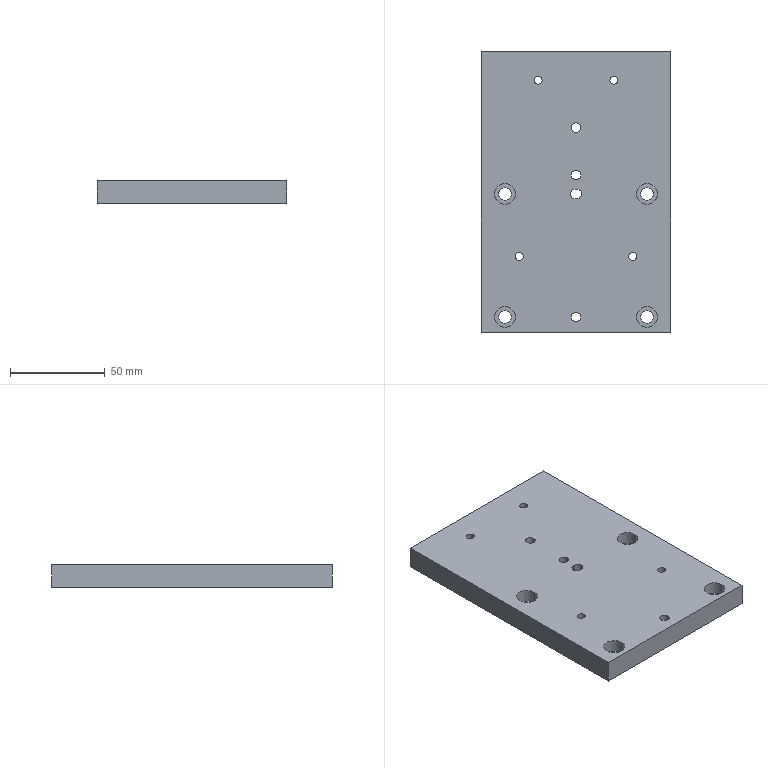Part | SolidWorks | features HoleWzd 6, Extrusion 1 | 1 solid | 45 faces | box 100 x 148 x 12 mm | volume 172636 mm3 | cylinder 33 | plane 12 | commonest cylinder face diameters 5 x9 4.2 x8 6.6 x8 11 x8
STEP:
#1=CARTESIAN_POINT('',(-32.1,-34.,0.));
#2=VERTEX_POINT('',#1);
#3=CARTESIAN_POINT('',(-27.9,-34.,0.));
#4=VERTEX_POINT('',#3);
#5=CARTESIAN_POINT('',(-30.,-34.,0.));
#6=DIRECTION('',(0.,0.,1.));
#7=DIRECTION('',(1.,0.,0.));
#8=AXIS2_PLACEMENT_3D('',#5,#6,#7);
#9=CIRCLE('',#8,2.1);
#10=EDGE_CURVE('',#2,#4,#9,.T.);
#11=ORIENTED_EDGE('',*,*,#10,.F.);
#12=CARTESIAN_POINT('',(-32.1,-34.,12.));
#13=VERTEX_POINT('',#12);
#14=CARTESIAN_POINT('',(-32.1,-34.,12.));
#15=DIRECTION('',(0.,0.,1.));
#16=VECTOR('',#15,1000.);
#17=LINE('',#14,#16);
#18=EDGE_CURVE('',#2,#13,#17,.T.);
#19=ORIENTED_EDGE('',*,*,#18,.T.);
#20=CARTESIAN_POINT('',(-27.9,-34.,12.));
#21=VERTEX_POINT('',#20);
#22=CARTESIAN_POINT('',(-30.,-34.,12.));
#23=DIRECTION('',(0.,0.,1.));
#24=DIRECTION('',(1.,0.,0.));
#25=AXIS2_PLACEMENT_3D('',#22,#23,#24);
#26=CIRCLE('',#25,2.1);
#27=EDGE_CURVE('',#13,#21,#26,.T.);
#28=ORIENTED_EDGE('',*,*,#27,.T.);
#29=CARTESIAN_POINT('',(-27.9,-34.,12.));
#30=DIRECTION('',(0.,0.,1.));
#31=VECTOR('',#30,1000.);
#32=LINE('',#29,#31);
#33=EDGE_CURVE('',#4,#21,#32,.T.);
#34=ORIENTED_EDGE('',*,*,#33,.F.);
#35=EDGE_LOOP('',(#11,#19,#28,#34));
#36=FACE_OUTER_BOUND('',#35,.T.);
#37=CARTESIAN_POINT('',(-30.,-34.,12.));
#38=DIRECTION('',(0.,0.,1.));
#39=DIRECTION('',(1.,0.,0.));
#40=AXIS2_PLACEMENT_3D('',#37,#38,#39);
#41=CYLINDRICAL_SURFACE('',#40,2.1);
#42=ADVANCED_FACE('',(#36),#41,.F.);
#43=CARTESIAN_POINT('',(27.9,-34.,0.));
#44=VERTEX_POINT('',#43);
#45=CARTESIAN_POINT('',(32.1,-34.,0.));
#46=VERTEX_POINT('',#45);
#47=CARTESIAN_POINT('',(30.,-34.,0.));
#48=DIRECTION('',(0.,0.,1.));
#49=DIRECTION('',(1.,0.,0.));
#50=AXIS2_PLACEMENT_3D('',#47,#48,#49);
#51=CIRCLE('',#50,2.1);
#52=EDGE_CURVE('',#44,#46,#51,.T.);
#53=ORIENTED_EDGE('',*,*,#52,.F.);
#54=CARTESIAN_POINT('',(27.9,-34.,12.));
#55=VERTEX_POINT('',#54);
#56=CARTESIAN_POINT('',(27.9,-34.,12.));
#57=DIRECTION('',(0.,0.,1.));
#58=VECTOR('',#57,1000.);
#59=LINE('',#56,#58);
#60=EDGE_CURVE('',#44,#55,#59,.T.);
#61=ORIENTED_EDGE('',*,*,#60,.T.);
#62=CARTESIAN_POINT('',(32.1,-34.,12.));
#63=VERTEX_POINT('',#62);
#64=CARTESIAN_POINT('',(30.,-34.,12.));
#65=DIRECTION('',(0.,0.,1.));
#66=DIRECTION('',(1.,0.,0.));
#67=AXIS2_PLACEMENT_3D('',#64,#65,#66);
#68=CIRCLE('',#67,2.1);
#69=EDGE_CURVE('',#55,#63,#68,.T.);
#70=ORIENTED_EDGE('',*,*,#69,.T.);
#71=CARTESIAN_POINT('',(32.1,-34.,12.));
#72=DIRECTION('',(0.,0.,1.));
#73=VECTOR('',#72,1000.);
#74=LINE('',#71,#73);
#75=EDGE_CURVE('',#46,#63,#74,.T.);
#76=ORIENTED_EDGE('',*,*,#75,.F.);
#77=EDGE_LOOP('',(#53,#61,#70,#76));
#78=FACE_OUTER_BOUND('',#77,.T.);
#79=CARTESIAN_POINT('',(30.,-34.,12.));
#80=DIRECTION('',(0.,0.,1.));
#81=DIRECTION('',(1.,0.,0.));
#82=AXIS2_PLACEMENT_3D('',#79,#80,#81);
#83=CYLINDRICAL_SURFACE('',#82,2.1);
#84=ADVANCED_FACE('',(#78),#83,.F.);
#85=CARTESIAN_POINT('',(-2.5,34.,0.));
#86=VERTEX_POINT('',#85);
#87=CARTESIAN_POINT('',(2.5,34.,0.));
#88=VERTEX_POINT('',#87);
#89=CARTESIAN_POINT('',(0.,34.,0.));
#90=DIRECTION('',(0.,0.,1.));
#91=DIRECTION('',(1.,0.,0.));
#92=AXIS2_PLACEMENT_3D('',#89,#90,#91);
#93=CIRCLE('',#92,2.5);
#94=EDGE_CURVE('',#86,#88,#93,.T.);
#95=ORIENTED_EDGE('',*,*,#94,.F.);
#96=CARTESIAN_POINT('',(-2.5,34.,12.));
#97=VERTEX_POINT('',#96);
#98=CARTESIAN_POINT('',(-2.5,34.,12.));
#99=DIRECTION('',(0.,0.,1.));
#100=VECTOR('',#99,1000.);
#101=LINE('',#98,#100);
#102=EDGE_CURVE('',#86,#97,#101,.T.);
#103=ORIENTED_EDGE('',*,*,#102,.T.);
#104=CARTESIAN_POINT('',(2.5,34.,12.));
#105=VERTEX_POINT('',#104);
#106=CARTESIAN_POINT('',(0.,34.,12.));
#107=DIRECTION('',(0.,0.,1.));
#108=DIRECTION('',(1.,0.,0.));
#109=AXIS2_PLACEMENT_3D('',#106,#107,#108);
#110=CIRCLE('',#109,2.5);
#111=EDGE_CURVE('',#97,#105,#110,.T.);
#112=ORIENTED_EDGE('',*,*,#111,.T.);
#113=CARTESIAN_POINT('',(2.5,34.,12.));
#114=DIRECTION('',(0.,0.,1.));
#115=VECTOR('',#114,1000.);
#116=LINE('',#113,#115);
#117=EDGE_CURVE('',#88,#105,#116,.T.);
#118=ORIENTED_EDGE('',*,*,#117,.F.);
#119=EDGE_LOOP('',(#95,#103,#112,#118));
#120=FACE_OUTER_BOUND('',#119,.T.);
#121=CARTESIAN_POINT('',(0.,34.,12.));
#122=DIRECTION('',(0.,0.,1.));
#123=DIRECTION('',(1.,0.,0.));
#124=AXIS2_PLACEMENT_3D('',#121,#122,#123);
#125=CYLINDRICAL_SURFACE('',#124,2.5);
#126=ADVANCED_FACE('',(#120),#125,.F.);
#127=CARTESIAN_POINT('',(-2.5,9.,0.));
#128=VERTEX_POINT('',#127);
#129=CARTESIAN_POINT('',(2.5,9.,0.));
#130=VERTEX_POINT('',#129);
#131=CARTESIAN_POINT('',(0.,9.,0.));
#132=DIRECTION('',(0.,0.,1.));
#133=DIRECTION('',(1.,0.,0.));
#134=AXIS2_PLACEMENT_3D('',#131,#132,#133);
#135=CIRCLE('',#134,2.5);
#136=EDGE_CURVE('',#128,#130,#135,.T.);
#137=ORIENTED_EDGE('',*,*,#136,.F.);
#138=CARTESIAN_POINT('',(-2.5,9.,12.));
#139=VERTEX_POINT('',#138);
#140=CARTESIAN_POINT('',(-2.5,9.,12.));
#141=DIRECTION('',(0.,0.,1.));
#142=VECTOR('',#141,1000.);
#143=LINE('',#140,#142);
#144=EDGE_CURVE('',#128,#139,#143,.T.);
#145=ORIENTED_EDGE('',*,*,#144,.T.);
#146=CARTESIAN_POINT('',(2.5,9.,12.));
#147=VERTEX_POINT('',#146);
#148=CARTESIAN_POINT('',(0.,9.,12.));
#149=DIRECTION('',(0.,0.,1.));
#150=DIRECTION('',(1.,0.,0.));
#151=AXIS2_PLACEMENT_3D('',#148,#149,#150);
#152=CIRCLE('',#151,2.5);
#153=EDGE_CURVE('',#139,#147,#152,.T.);
#154=ORIENTED_EDGE('',*,*,#153,.T.);
#155=CARTESIAN_POINT('',(2.5,9.,12.));
#156=DIRECTION('',(0.,0.,1.));
#157=VECTOR('',#156,1000.);
#158=LINE('',#155,#157);
#159=EDGE_CURVE('',#130,#147,#158,.T.);
#160=ORIENTED_EDGE('',*,*,#159,.F.);
#161=EDGE_LOOP('',(#137,#145,#154,#160));
#162=FACE_OUTER_BOUND('',#161,.T.);
#163=CARTESIAN_POINT('',(0.,9.,12.));
#164=DIRECTION('',(0.,0.,1.));
#165=DIRECTION('',(1.,0.,0.));
#166=AXIS2_PLACEMENT_3D('',#163,#164,#165);
#167=CYLINDRICAL_SURFACE('',#166,2.5);
#168=ADVANCED_FACE('',(#162),#167,.F.);
#169=CARTESIAN_POINT('',(22.1,59.,12.));
#170=VERTEX_POINT('',#169);
#171=CARTESIAN_POINT('',(17.9,59.,12.));
#172=VERTEX_POINT('',#171);
#173=CARTESIAN_POINT('',(20.,59.,12.));
#174=DIRECTION('',(0.,0.,-1.));
#175=DIRECTION('',(-1.,0.,0.));
#176=AXIS2_PLACEMENT_3D('',#173,#174,#175);
#177=CIRCLE('',#176,2.1);
#178=EDGE_CURVE('',#170,#172,#177,.T.);
#179=ORIENTED_EDGE('',*,*,#178,.F.);
#180=CARTESIAN_POINT('',(22.1,59.,0.));
#181=VERTEX_POINT('',#180);
#182=CARTESIAN_POINT('',(22.1,59.,0.));
#183=DIRECTION('',(0.,0.,-1.));
#184=VECTOR('',#183,1000.);
#185=LINE('',#182,#184);
#186=EDGE_CURVE('',#170,#181,#185,.T.);
#187=ORIENTED_EDGE('',*,*,#186,.T.);
#188=CARTESIAN_POINT('',(17.9,59.,0.));
#189=VERTEX_POINT('',#188);
#190=CARTESIAN_POINT('',(20.,59.,0.));
#191=DIRECTION('',(0.,0.,-1.));
#192=DIRECTION('',(-1.,0.,0.));
#193=AXIS2_PLACEMENT_3D('',#190,#191,#192);
#194=CIRCLE('',#193,2.1);
#195=EDGE_CURVE('',#181,#189,#194,.T.);
#196=ORIENTED_EDGE('',*,*,#195,.T.);
#197=CARTESIAN_POINT('',(17.9,59.,0.));
#198=DIRECTION('',(0.,0.,-1.));
#199=VECTOR('',#198,1000.);
#200=LINE('',#197,#199);
#201=EDGE_CURVE('',#172,#189,#200,.T.);
#202=ORIENTED_EDGE('',*,*,#201,.F.);
#203=EDGE_LOOP('',(#179,#187,#196,#202));
#204=FACE_OUTER_BOUND('',#203,.T.);
#205=CARTESIAN_POINT('',(20.,59.,0.));
#206=DIRECTION('',(0.,0.,-1.));
#207=DIRECTION('',(-1.,0.,0.));
#208=AXIS2_PLACEMENT_3D('',#205,#206,#207);
#209=CYLINDRICAL_SURFACE('',#208,2.1);
#210=ADVANCED_FACE('',(#204),#209,.F.);
#211=CARTESIAN_POINT('',(-17.9,59.,12.));
#212=VERTEX_POINT('',#211);
#213=CARTESIAN_POINT('',(-22.1,59.,12.));
#214=VERTEX_POINT('',#213);
#215=CARTESIAN_POINT('',(-20.,59.,12.));
#216=DIRECTION('',(0.,0.,-1.));
#217=DIRECTION('',(-1.,0.,0.));
#218=AXIS2_PLACEMENT_3D('',#215,#216,#217);
#219=CIRCLE('',#218,2.1);
#220=EDGE_CURVE('',#212,#214,#219,.T.);
#221=ORIENTED_EDGE('',*,*,#220,.F.);
#222=CARTESIAN_POINT('',(-17.9,59.,0.));
#223=VERTEX_POINT('',#222);
#224=CARTESIAN_POINT('',(-17.9,59.,0.));
#225=DIRECTION('',(0.,0.,-1.));
#226=VECTOR('',#225,1000.);
#227=LINE('',#224,#226);
#228=EDGE_CURVE('',#212,#223,#227,.T.);
#229=ORIENTED_EDGE('',*,*,#228,.T.);
#230=CARTESIAN_POINT('',(-22.1,59.,0.));
#231=VERTEX_POINT('',#230);
#232=CARTESIAN_POINT('',(-20.,59.,0.));
#233=DIRECTION('',(0.,0.,-1.));
#234=DIRECTION('',(-1.,0.,0.));
#235=AXIS2_PLACEMENT_3D('',#232,#233,#234);
#236=CIRCLE('',#235,2.1);
#237=EDGE_CURVE('',#223,#231,#236,.T.);
#238=ORIENTED_EDGE('',*,*,#237,.T.);
#239=CARTESIAN_POINT('',(-22.1,59.,0.));
#240=DIRECTION('',(0.,0.,-1.));
#241=VECTOR('',#240,1000.);
#242=LINE('',#239,#241);
#243=EDGE_CURVE('',#214,#231,#242,.T.);
#244=ORIENTED_EDGE('',*,*,#243,.F.);
#245=EDGE_LOOP('',(#221,#229,#238,#244));
#246=FACE_OUTER_BOUND('',#245,.T.);
#247=CARTESIAN_POINT('',(-20.,59.,0.));
#248=DIRECTION('',(0.,0.,-1.));
#249=DIRECTION('',(-1.,0.,0.));
#250=AXIS2_PLACEMENT_3D('',#247,#248,#249);
#251=CYLINDRICAL_SURFACE('',#250,2.1);
#252=ADVANCED_FACE('',(#246),#251,.F.);
#253=CARTESIAN_POINT('',(3.,-1.,0.));
#254=VERTEX_POINT('',#253);
#255=CARTESIAN_POINT('',(0.5,1.5,0.));
#256=VERTEX_POINT('',#255);
#257=CARTESIAN_POINT('',(0.5,-1.,0.));
#258=DIRECTION('',(0.,0.,1.));
#259=DIRECTION('',(1.,0.,0.));
#260=AXIS2_PLACEMENT_3D('',#257,#258,#259);
#261=CIRCLE('',#260,2.5);
#262=EDGE_CURVE('',#254,#256,#261,.T.);
#263=ORIENTED_EDGE('',*,*,#262,.F.);
#264=CARTESIAN_POINT('',(3.,-1.,12.));
#265=VERTEX_POINT('',#264);
#266=CARTESIAN_POINT('',(3.,-1.,12.));
#267=DIRECTION('',(0.,0.,1.));
#268=VECTOR('',#267,1000.);
#269=LINE('',#266,#268);
#270=EDGE_CURVE('',#254,#265,#269,.T.);
#271=ORIENTED_EDGE('',*,*,#270,.T.);
#272=CARTESIAN_POINT('',(0.5,1.5,12.));
#273=VERTEX_POINT('',#272);
#274=CARTESIAN_POINT('',(0.5,-1.,12.));
#275=DIRECTION('',(0.,0.,1.));
#276=DIRECTION('',(1.,0.,0.));
#277=AXIS2_PLACEMENT_3D('',#274,#275,#276);
#278=CIRCLE('',#277,2.5);
#279=EDGE_CURVE('',#265,#273,#278,.T.);
#280=ORIENTED_EDGE('',*,*,#279,.T.);
#281=CARTESIAN_POINT('',(0.5,1.5,12.));
#282=DIRECTION('',(0.,0.,1.));
#283=VECTOR('',#282,1000.);
#284=LINE('',#281,#283);
#285=EDGE_CURVE('',#256,#273,#284,.T.);
#286=ORIENTED_EDGE('',*,*,#285,.F.);
#287=EDGE_LOOP('',(#263,#271,#280,#286));
#288=FACE_OUTER_BOUND('',#287,.T.);
#289=CARTESIAN_POINT('',(0.5,-1.,12.));
#290=DIRECTION('',(0.,0.,1.));
#291=DIRECTION('',(1.,0.,0.));
#292=AXIS2_PLACEMENT_3D('',#289,#290,#291);
#293=CYLINDRICAL_SURFACE('',#292,2.5);
#294=ADVANCED_FACE('',(#288),#293,.F.);
#295=CARTESIAN_POINT('',(-2.5,-66.,0.));
#296=VERTEX_POINT('',#295);
#297=CARTESIAN_POINT('',(2.5,-66.,0.));
#298=VERTEX_POINT('',#297);
#299=CARTESIAN_POINT('',(0.,-66.,0.));
#300=DIRECTION('',(0.,0.,1.));
#301=DIRECTION('',(1.,0.,0.));
#302=AXIS2_PLACEMENT_3D('',#299,#300,#301);
#303=CIRCLE('',#302,2.5);
#304=EDGE_CURVE('',#296,#298,#303,.T.);
#305=ORIENTED_EDGE('',*,*,#304,.F.);
#306=CARTESIAN_POINT('',(-2.5,-66.,12.));
#307=VERTEX_POINT('',#306);
#308=CARTESIAN_POINT('',(-2.5,-66.,12.));
#309=DIRECTION('',(0.,0.,1.));
#310=VECTOR('',#309,1000.);
#311=LINE('',#308,#310);
#312=EDGE_CURVE('',#296,#307,#311,.T.);
#313=ORIENTED_EDGE('',*,*,#312,.T.);
#314=CARTESIAN_POINT('',(2.5,-66.,12.));
#315=VERTEX_POINT('',#314);
#316=CARTESIAN_POINT('',(0.,-66.,12.));
#317=DIRECTION('',(0.,0.,1.));
#318=DIRECTION('',(1.,0.,0.));
#319=AXIS2_PLACEMENT_3D('',#316,#317,#318);
#320=CIRCLE('',#319,2.5);
#321=EDGE_CURVE('',#307,#315,#320,.T.);
#322=ORIENTED_EDGE('',*,*,#321,.T.);
#323=CARTESIAN_POINT('',(2.5,-66.,12.));
#324=DIRECTION('',(0.,0.,1.));
#325=VECTOR('',#324,1000.);
#326=LINE('',#323,#325);
#327=EDGE_CURVE('',#298,#315,#326,.T.);
#328=ORIENTED_EDGE('',*,*,#327,.F.);
#329=EDGE_LOOP('',(#305,#313,#322,#328));
#330=FACE_OUTER_BOUND('',#329,.T.);
#331=CARTESIAN_POINT('',(0.,-66.,12.));
#332=DIRECTION('',(0.,0.,1.));
#333=DIRECTION('',(1.,0.,0.));
#334=AXIS2_PLACEMENT_3D('',#331,#332,#333);
#335=CYLINDRICAL_SURFACE('',#334,2.5);
#336=ADVANCED_FACE('',(#330),#335,.F.);
#337=CARTESIAN_POINT('',(-43.,-1.,5.2));
#338=VERTEX_POINT('',#337);
#339=CARTESIAN_POINT('',(-32.,-1.,5.2));
#340=VERTEX_POINT('',#339);
#341=CARTESIAN_POINT('',(-37.5,-1.,5.2));
#342=DIRECTION('',(0.,0.,1.));
#343=DIRECTION('',(1.,0.,0.));
#344=AXIS2_PLACEMENT_3D('',#341,#342,#343);
#345=CIRCLE('',#344,5.5);
#346=EDGE_CURVE('',#338,#340,#345,.T.);
#347=ORIENTED_EDGE('',*,*,#346,.F.);
#348=CARTESIAN_POINT('',(-43.,-1.,12.));
#349=VERTEX_POINT('',#348);
#350=CARTESIAN_POINT('',(-43.,-1.,12.));
#351=DIRECTION('',(0.,0.,1.));
#352=VECTOR('',#351,1000.);
#353=LINE('',#350,#352);
#354=EDGE_CURVE('',#338,#349,#353,.T.);
#355=ORIENTED_EDGE('',*,*,#354,.T.);
#356=CARTESIAN_POINT('',(-32.,-1.,12.));
#357=VERTEX_POINT('',#356);
#358=CARTESIAN_POINT('',(-37.5,-1.,12.));
#359=DIRECTION('',(0.,0.,1.));
#360=DIRECTION('',(1.,0.,0.));
#361=AXIS2_PLACEMENT_3D('',#358,#359,#360);
#362=CIRCLE('',#361,5.5);
#363=EDGE_CURVE('',#349,#357,#362,.T.);
#364=ORIENTED_EDGE('',*,*,#363,.T.);
#365=CARTESIAN_POINT('',(-32.,-1.,12.));
#366=DIRECTION('',(0.,0.,1.));
#367=VECTOR('',#366,1000.);
#368=LINE('',#365,#367);
#369=EDGE_CURVE('',#340,#357,#368,.T.);
#370=ORIENTED_EDGE('',*,*,#369,.F.);
#371=EDGE_LOOP('',(#347,#355,#364,#370));
#372=FACE_OUTER_BOUND('',#371,.T.);
#373=CARTESIAN_POINT('',(-37.5,-1.,12.));
#374=DIRECTION('',(0.,0.,1.));
#375=DIRECTION('',(1.,0.,0.));
#376=AXIS2_PLACEMENT_3D('',#373,#374,#375);
#377=CYLINDRICAL_SURFACE('',#376,5.5);
#378=ADVANCED_FACE('',(#372),#377,.F.);
#379=CARTESIAN_POINT('',(-40.8,-1.,0.));
#380=VERTEX_POINT('',#379);
#381=CARTESIAN_POINT('',(-34.2,-1.,0.));
#382=VERTEX_POINT('',#381);
#383=CARTESIAN_POINT('',(-37.5,-1.,0.));
#384=DIRECTION('',(0.,0.,1.));
#385=DIRECTION('',(1.,0.,0.));
#386=AXIS2_PLACEMENT_3D('',#383,#384,#385);
#387=CIRCLE('',#386,3.3);
#388=EDGE_CURVE('',#380,#382,#387,.T.);
#389=ORIENTED_EDGE('',*,*,#388,.F.);
#390=CARTESIAN_POINT('',(-40.8,-1.,5.2));
#391=VERTEX_POINT('',#390);
#392=CARTESIAN_POINT('',(-40.8,-1.,12.));
#393=DIRECTION('',(0.,0.,1.));
#394=VECTOR('',#393,1000.);
#395=LINE('',#392,#394);
#396=EDGE_CURVE('',#380,#391,#395,.T.);
#397=ORIENTED_EDGE('',*,*,#396,.T.);
#398=CARTESIAN_POINT('',(-34.2,-1.,5.2));
#399=VERTEX_POINT('',#398);
#400=CARTESIAN_POINT('',(-37.5,-1.,5.2));
#401=DIRECTION('',(0.,0.,1.));
#402=DIRECTION('',(1.,0.,0.));
#403=AXIS2_PLACEMENT_3D('',#400,#401,#402);
#404=CIRCLE('',#403,3.3);
#405=EDGE_CURVE('',#391,#399,#404,.T.);
#406=ORIENTED_EDGE('',*,*,#405,.T.);
#407=CARTESIAN_POINT('',(-34.2,-1.,12.));
#408=DIRECTION('',(0.,0.,1.));
#409=VECTOR('',#408,1000.);
#410=LINE('',#407,#409);
#411=EDGE_CURVE('',#382,#399,#410,.T.);
#412=ORIENTED_EDGE('',*,*,#411,.F.);
#413=EDGE_LOOP('',(#389,#397,#406,#412));
#414=FACE_OUTER_BOUND('',#413,.T.);
#415=CARTESIAN_POINT('',(-37.5,-1.,12.));
#416=DIRECTION('',(0.,0.,1.));
#417=DIRECTION('',(1.,0.,0.));
#418=AXIS2_PLACEMENT_3D('',#415,#416,#417);
#419=CYLINDRICAL_SURFACE('',#418,3.3);
#420=ADVANCED_FACE('',(#414),#419,.F.);
#421=CARTESIAN_POINT('',(-43.,-66.,5.2));
#422=VERTEX_POINT('',#421);
#423=CARTESIAN_POINT('',(-32.,-66.,5.2));
#424=VERTEX_POINT('',#423);
#425=CARTESIAN_POINT('',(-37.5,-66.,5.2));
#426=DIRECTION('',(0.,0.,1.));
#427=DIRECTION('',(1.,0.,0.));
#428=AXIS2_PLACEMENT_3D('',#425,#426,#427);
#429=CIRCLE('',#428,5.5);
#430=EDGE_CURVE('',#422,#424,#429,.T.);
#431=ORIENTED_EDGE('',*,*,#430,.F.);
#432=CARTESIAN_POINT('',(-43.,-66.,12.));
#433=VERTEX_POINT('',#432);
#434=CARTESIAN_POINT('',(-43.,-66.,12.));
#435=DIRECTION('',(0.,0.,1.));
#436=VECTOR('',#435,1000.);
#437=LINE('',#434,#436);
#438=EDGE_CURVE('',#422,#433,#437,.T.);
#439=ORIENTED_EDGE('',*,*,#438,.T.);
#440=CARTESIAN_POINT('',(-32.,-66.,12.));
#441=VERTEX_POINT('',#440);
#442=CARTESIAN_POINT('',(-37.5,-66.,12.));
#443=DIRECTION('',(0.,0.,1.));
#444=DIRECTION('',(1.,0.,0.));
#445=AXIS2_PLACEMENT_3D('',#442,#443,#444);
#446=CIRCLE('',#445,5.5);
#447=EDGE_CURVE('',#433,#441,#446,.T.);
#448=ORIENTED_EDGE('',*,*,#447,.T.);
#449=CARTESIAN_POINT('',(-32.,-66.,12.));
#450=DIRECTION('',(0.,0.,1.));
#451=VECTOR('',#450,1000.);
#452=LINE('',#449,#451);
#453=EDGE_CURVE('',#424,#441,#452,.T.);
#454=ORIENTED_EDGE('',*,*,#453,.F.);
#455=EDGE_LOOP('',(#431,#439,#448,#454));
#456=FACE_OUTER_BOUND('',#455,.T.);
#457=CARTESIAN_POINT('',(-37.5,-66.,12.));
#458=DIRECTION('',(0.,0.,1.));
#459=DIRECTION('',(1.,0.,0.));
#460=AXIS2_PLACEMENT_3D('',#457,#458,#459);
#461=CYLINDRICAL_SURFACE('',#460,5.5);
#462=ADVANCED_FACE('',(#456),#461,.F.);
#463=CARTESIAN_POINT('',(-40.8,-66.,0.));
#464=VERTEX_POINT('',#463);
#465=CARTESIAN_POINT('',(-34.2,-66.,0.));
#466=VERTEX_POINT('',#465);
#467=CARTESIAN_POINT('',(-37.5,-66.,0.));
#468=DIRECTION('',(0.,0.,1.));
#469=DIRECTION('',(1.,0.,0.));
#470=AXIS2_PLACEMENT_3D('',#467,#468,#469);
#471=CIRCLE('',#470,3.3);
#472=EDGE_CURVE('',#464,#466,#471,.T.);
#473=ORIENTED_EDGE('',*,*,#472,.F.);
#474=CARTESIAN_POINT('',(-40.8,-66.,5.2));
#475=VERTEX_POINT('',#474);
#476=CARTESIAN_POINT('',(-40.8,-66.,12.));
#477=DIRECTION('',(0.,0.,1.));
#478=VECTOR('',#477,1000.);
#479=LINE('',#476,#478);
#480=EDGE_CURVE('',#464,#475,#479,.T.);
#481=ORIENTED_EDGE('',*,*,#480,.T.);
#482=CARTESIAN_POINT('',(-34.2,-66.,5.2));
#483=VERTEX_POINT('',#482);
#484=CARTESIAN_POINT('',(-37.5,-66.,5.2));
#485=DIRECTION('',(0.,0.,1.));
#486=DIRECTION('',(1.,0.,0.));
#487=AXIS2_PLACEMENT_3D('',#484,#485,#486);
#488=CIRCLE('',#487,3.3);
#489=EDGE_CURVE('',#475,#483,#488,.T.);
#490=ORIENTED_EDGE('',*,*,#489,.T.);
#491=CARTESIAN_POINT('',(-34.2,-66.,12.));
#492=DIRECTION('',(0.,0.,1.));
#493=VECTOR('',#492,1000.);
#494=LINE('',#491,#493);
#495=EDGE_CURVE('',#466,#483,#494,.T.);
#496=ORIENTED_EDGE('',*,*,#495,.F.);
#497=EDGE_LOOP('',(#473,#481,#490,#496));
#498=FACE_OUTER_BOUND('',#497,.T.);
#499=CARTESIAN_POINT('',(-37.5,-66.,12.));
#500=DIRECTION('',(0.,0.,1.));
#501=DIRECTION('',(1.,0.,0.));
#502=AXIS2_PLACEMENT_3D('',#499,#500,#501);
#503=CYLINDRICAL_SURFACE('',#502,3.3);
#504=ADVANCED_FACE('',(#498),#503,.F.);
#505=CARTESIAN_POINT('',(32.,-1.,5.2));
#506=VERTEX_POINT('',#505);
#507=CARTESIAN_POINT('',(43.,-1.,5.2));
#508=VERTEX_POINT('',#507);
#509=CARTESIAN_POINT('',(37.5,-1.,5.2));
#510=DIRECTION('',(0.,0.,1.));
#511=DIRECTION('',(1.,0.,0.));
#512=AXIS2_PLACEMENT_3D('',#509,#510,#511);
#513=CIRCLE('',#512,5.5);
#514=EDGE_CURVE('',#506,#508,#513,.T.);
#515=ORIENTED_EDGE('',*,*,#514,.F.);
#516=CARTESIAN_POINT('',(32.,-1.,12.));
#517=VERTEX_POINT('',#516);
#518=CARTESIAN_POINT('',(32.,-1.,12.));
#519=DIRECTION('',(0.,0.,1.));
#520=VECTOR('',#519,1000.);
#521=LINE('',#518,#520);
#522=EDGE_CURVE('',#506,#517,#521,.T.);
#523=ORIENTED_EDGE('',*,*,#522,.T.);
#524=CARTESIAN_POINT('',(43.,-1.,12.));
#525=VERTEX_POINT('',#524);
#526=CARTESIAN_POINT('',(37.5,-1.,12.));
#527=DIRECTION('',(0.,0.,1.));
#528=DIRECTION('',(1.,0.,0.));
#529=AXIS2_PLACEMENT_3D('',#526,#527,#528);
#530=CIRCLE('',#529,5.5);
#531=EDGE_CURVE('',#517,#525,#530,.T.);
#532=ORIENTED_EDGE('',*,*,#531,.T.);
#533=CARTESIAN_POINT('',(43.,-1.,12.));
#534=DIRECTION('',(0.,0.,1.));
#535=VECTOR('',#534,1000.);
#536=LINE('',#533,#535);
#537=EDGE_CURVE('',#508,#525,#536,.T.);
#538=ORIENTED_EDGE('',*,*,#537,.F.);
#539=EDGE_LOOP('',(#515,#523,#532,#538));
#540=FACE_OUTER_BOUND('',#539,.T.);
#541=CARTESIAN_POINT('',(37.5,-1.,12.));
#542=DIRECTION('',(0.,0.,1.));
#543=DIRECTION('',(1.,0.,0.));
#544=AXIS2_PLACEMENT_3D('',#541,#542,#543);
#545=CYLINDRICAL_SURFACE('',#544,5.5);
#546=ADVANCED_FACE('',(#540),#545,.F.);
#547=CARTESIAN_POINT('',(34.2,-1.,0.));
#548=VERTEX_POINT('',#547);
#549=CARTESIAN_POINT('',(40.8,-1.,0.));
#550=VERTEX_POINT('',#549);
#551=CARTESIAN_POINT('',(37.5,-1.,0.));
#552=DIRECTION('',(0.,0.,1.));
#553=DIRECTION('',(1.,0.,0.));
#554=AXIS2_PLACEMENT_3D('',#551,#552,#553);
#555=CIRCLE('',#554,3.3);
#556=EDGE_CURVE('',#548,#550,#555,.T.);
#557=ORIENTED_EDGE('',*,*,#556,.F.);
#558=CARTESIAN_POINT('',(34.2,-1.,5.2));
#559=VERTEX_POINT('',#558);
#560=CARTESIAN_POINT('',(34.2,-1.,12.));
#561=DIRECTION('',(0.,0.,1.));
#562=VECTOR('',#561,1000.);
#563=LINE('',#560,#562);
#564=EDGE_CURVE('',#548,#559,#563,.T.);
#565=ORIENTED_EDGE('',*,*,#564,.T.);
#566=CARTESIAN_POINT('',(40.8,-1.,5.2));
#567=VERTEX_POINT('',#566);
#568=CARTESIAN_POINT('',(37.5,-1.,5.2));
#569=DIRECTION('',(0.,0.,1.));
#570=DIRECTION('',(1.,0.,0.));
#571=AXIS2_PLACEMENT_3D('',#568,#569,#570);
#572=CIRCLE('',#571,3.3);
#573=EDGE_CURVE('',#559,#567,#572,.T.);
#574=ORIENTED_EDGE('',*,*,#573,.T.);
#575=CARTESIAN_POINT('',(40.8,-1.,12.));
#576=DIRECTION('',(0.,0.,1.));
#577=VECTOR('',#576,1000.);
#578=LINE('',#575,#577);
#579=EDGE_CURVE('',#550,#567,#578,.T.);
#580=ORIENTED_EDGE('',*,*,#579,.F.);
#581=EDGE_LOOP('',(#557,#565,#574,#580));
#582=FACE_OUTER_BOUND('',#581,.T.);
#583=CARTESIAN_POINT('',(37.5,-1.,12.));
#584=DIRECTION('',(0.,0.,1.));
#585=DIRECTION('',(1.,0.,0.));
#586=AXIS2_PLACEMENT_3D('',#583,#584,#585);
#587=CYLINDRICAL_SURFACE('',#586,3.3);
#588=ADVANCED_FACE('',(#582),#587,.F.);
#589=CARTESIAN_POINT('',(32.,-66.,5.2));
#590=VERTEX_POINT('',#589);
#591=CARTESIAN_POINT('',(43.,-66.,5.2));
#592=VERTEX_POINT('',#591);
#593=CARTESIAN_POINT('',(37.5,-66.,5.2));
#594=DIRECTION('',(0.,0.,1.));
#595=DIRECTION('',(1.,0.,0.));
#596=AXIS2_PLACEMENT_3D('',#593,#594,#595);
#597=CIRCLE('',#596,5.5);
#598=EDGE_CURVE('',#590,#592,#597,.T.);
#599=ORIENTED_EDGE('',*,*,#598,.F.);
#600=CARTESIAN_POINT('',(32.,-66.,12.));
#601=VERTEX_POINT('',#600);
#602=CARTESIAN_POINT('',(32.,-66.,12.));
#603=DIRECTION('',(0.,0.,1.));
#604=VECTOR('',#603,1000.);
#605=LINE('',#602,#604);
#606=EDGE_CURVE('',#590,#601,#605,.T.);
#607=ORIENTED_EDGE('',*,*,#606,.T.);
#608=CARTESIAN_POINT('',(43.,-66.,12.));
#609=VERTEX_POINT('',#608);
#610=CARTESIAN_POINT('',(37.5,-66.,12.));
#611=DIRECTION('',(0.,0.,1.));
#612=DIRECTION('',(1.,0.,0.));
#613=AXIS2_PLACEMENT_3D('',#610,#611,#612);
#614=CIRCLE('',#613,5.5);
#615=EDGE_CURVE('',#601,#609,#614,.T.);
#616=ORIENTED_EDGE('',*,*,#615,.T.);
#617=CARTESIAN_POINT('',(43.,-66.,12.));
#618=DIRECTION('',(0.,0.,1.));
#619=VECTOR('',#618,1000.);
#620=LINE('',#617,#619);
#621=EDGE_CURVE('',#592,#609,#620,.T.);
#622=ORIENTED_EDGE('',*,*,#621,.F.);
#623=EDGE_LOOP('',(#599,#607,#616,#622));
#624=FACE_OUTER_BOUND('',#623,.T.);
#625=CARTESIAN_POINT('',(37.5,-66.,12.));
#626=DIRECTION('',(0.,0.,1.));
#627=DIRECTION('',(1.,0.,0.));
#628=AXIS2_PLACEMENT_3D('',#625,#626,#627);
#629=CYLINDRICAL_SURFACE('',#628,5.5);
#630=ADVANCED_FACE('',(#624),#629,.F.);
#631=CARTESIAN_POINT('',(34.2,-66.,0.));
#632=VERTEX_POINT('',#631);
#633=CARTESIAN_POINT('',(40.8,-66.,0.));
#634=VERTEX_POINT('',#633);
#635=CARTESIAN_POINT('',(37.5,-66.,0.));
#636=DIRECTION('',(0.,0.,1.));
#637=DIRECTION('',(1.,0.,0.));
#638=AXIS2_PLACEMENT_3D('',#635,#636,#637);
#639=CIRCLE('',#638,3.3);
#640=EDGE_CURVE('',#632,#634,#639,.T.);
#641=ORIENTED_EDGE('',*,*,#640,.F.);
#642=CARTESIAN_POINT('',(34.2,-66.,5.2));
#643=VERTEX_POINT('',#642);
#644=CARTESIAN_POINT('',(34.2,-66.,12.));
#645=DIRECTION('',(0.,0.,1.));
#646=VECTOR('',#645,1000.);
#647=LINE('',#644,#646);
#648=EDGE_CURVE('',#632,#643,#647,.T.);
#649=ORIENTED_EDGE('',*,*,#648,.T.);
#650=CARTESIAN_POINT('',(40.8,-66.,5.2));
#651=VERTEX_POINT('',#650);
#652=CARTESIAN_POINT('',(37.5,-66.,5.2));
#653=DIRECTION('',(0.,0.,1.));
#654=DIRECTION('',(1.,0.,0.));
#655=AXIS2_PLACEMENT_3D('',#652,#653,#654);
#656=CIRCLE('',#655,3.3);
#657=EDGE_CURVE('',#643,#651,#656,.T.);
#658=ORIENTED_EDGE('',*,*,#657,.T.);
#659=CARTESIAN_POINT('',(40.8,-66.,12.));
#660=DIRECTION('',(0.,0.,1.));
#661=VECTOR('',#660,1000.);
#662=LINE('',#659,#661);
#663=EDGE_CURVE('',#634,#651,#662,.T.);
#664=ORIENTED_EDGE('',*,*,#663,.F.);
#665=EDGE_LOOP('',(#641,#649,#658,#664));
#666=FACE_OUTER_BOUND('',#665,.T.);
#667=CARTESIAN_POINT('',(37.5,-66.,12.));
#668=DIRECTION('',(0.,0.,1.));
#669=DIRECTION('',(1.,0.,0.));
#670=AXIS2_PLACEMENT_3D('',#667,#668,#669);
#671=CYLINDRICAL_SURFACE('',#670,3.3);
#672=ADVANCED_FACE('',(#666),#671,.F.);
#673=CARTESIAN_POINT('',(50.,-74.,0.));
#674=VERTEX_POINT('',#673);
#675=CARTESIAN_POINT('',(50.,74.,0.));
#676=VERTEX_POINT('',#675);
#677=CARTESIAN_POINT('',(50.,74.,0.));
#678=DIRECTION('',(0.,1.,0.));
#679=VECTOR('',#678,1000.);
#680=LINE('',#677,#679);
#681=EDGE_CURVE('',#674,#676,#680,.T.);
#682=ORIENTED_EDGE('',*,*,#681,.T.);
#683=CARTESIAN_POINT('',(50.,74.,12.));
#684=VERTEX_POINT('',#683);
#685=CARTESIAN_POINT('',(50.,74.,12.));
#686=DIRECTION('',(0.,0.,-1.));
#687=VECTOR('',#686,1000.);
#688=LINE('',#685,#687);
#689=EDGE_CURVE('',#684,#676,#688,.T.);
#690=ORIENTED_EDGE('',*,*,#689,.F.);
#691=CARTESIAN_POINT('',(50.,-74.,12.));
#692=VERTEX_POINT('',#691);
#693=CARTESIAN_POINT('',(50.,74.,12.));
#694=DIRECTION('',(0.,1.,0.));
#695=VECTOR('',#694,1000.);
#696=LINE('',#693,#695);
#697=EDGE_CURVE('',#692,#684,#696,.T.);
#698=ORIENTED_EDGE('',*,*,#697,.F.);
#699=CARTESIAN_POINT('',(50.,-74.,12.));
#700=DIRECTION('',(0.,0.,-1.));
#701=VECTOR('',#700,1000.);
#702=LINE('',#699,#701);
#703=EDGE_CURVE('',#692,#674,#702,.T.);
#704=ORIENTED_EDGE('',*,*,#703,.T.);
#705=EDGE_LOOP('',(#682,#690,#698,#704));
#706=FACE_OUTER_BOUND('',#705,.T.);
#707=CARTESIAN_POINT('',(50.,74.,12.));
#708=DIRECTION('',(-1.,0.,0.));
#709=DIRECTION('',(0.,-1.,0.));
#710=AXIS2_PLACEMENT_3D('',#707,#708,#709);
#711=PLANE('',#710);
#712=ADVANCED_FACE('',(#706),#711,.F.);
#713=CARTESIAN_POINT('',(-50.,74.,0.));
#714=VERTEX_POINT('',#713);
#715=CARTESIAN_POINT('',(-50.,74.,0.));
#716=DIRECTION('',(-1.,0.,0.));
#717=VECTOR('',#716,1000.);
#718=LINE('',#715,#717);
#719=EDGE_CURVE('',#676,#714,#718,.T.);
#720=ORIENTED_EDGE('',*,*,#719,.T.);
#721=CARTESIAN_POINT('',(-50.,74.,12.));
#722=VERTEX_POINT('',#721);
#723=CARTESIAN_POINT('',(-50.,74.,12.));
#724=DIRECTION('',(0.,0.,-1.));
#725=VECTOR('',#724,1000.);
#726=LINE('',#723,#725);
#727=EDGE_CURVE('',#722,#714,#726,.T.);
#728=ORIENTED_EDGE('',*,*,#727,.F.);
#729=CARTESIAN_POINT('',(-50.,74.,12.));
#730=DIRECTION('',(-1.,0.,0.));
#731=VECTOR('',#730,1000.);
#732=LINE('',#729,#731);
#733=EDGE_CURVE('',#684,#722,#732,.T.);
#734=ORIENTED_EDGE('',*,*,#733,.F.);
#735=ORIENTED_EDGE('',*,*,#689,.T.);
#736=EDGE_LOOP('',(#720,#728,#734,#735));
#737=FACE_OUTER_BOUND('',#736,.T.);
#738=CARTESIAN_POINT('',(-50.,74.,12.));
#739=DIRECTION('',(0.,-1.,0.));
#740=DIRECTION('',(1.,0.,0.));
#741=AXIS2_PLACEMENT_3D('',#738,#739,#740);
#742=PLANE('',#741);
#743=ADVANCED_FACE('',(#737),#742,.F.);
#744=CARTESIAN_POINT('',(-50.,-74.,0.));
#745=VERTEX_POINT('',#744);
#746=CARTESIAN_POINT('',(-50.,74.,0.));
#747=DIRECTION('',(0.,-1.,0.));
#748=VECTOR('',#747,1000.);
#749=LINE('',#746,#748);
#750=EDGE_CURVE('',#714,#745,#749,.T.);
#751=ORIENTED_EDGE('',*,*,#750,.T.);
#752=CARTESIAN_POINT('',(-50.,-74.,12.));
#753=VERTEX_POINT('',#752);
#754=CARTESIAN_POINT('',(-50.,-74.,12.));
#755=DIRECTION('',(0.,0.,-1.));
#756=VECTOR('',#755,1000.);
#757=LINE('',#754,#756);
#758=EDGE_CURVE('',#753,#745,#757,.T.);
#759=ORIENTED_EDGE('',*,*,#758,.F.);
#760=CARTESIAN_POINT('',(-50.,74.,12.));
#761=DIRECTION('',(0.,-1.,0.));
#762=VECTOR('',#761,1000.);
#763=LINE('',#760,#762);
#764=EDGE_CURVE('',#722,#753,#763,.T.);
#765=ORIENTED_EDGE('',*,*,#764,.F.);
#766=ORIENTED_EDGE('',*,*,#727,.T.);
#767=EDGE_LOOP('',(#751,#759,#765,#766));
#768=FACE_OUTER_BOUND('',#767,.T.);
#769=CARTESIAN_POINT('',(-50.,74.,12.));
#770=DIRECTION('',(1.,0.,0.));
#771=DIRECTION('',(0.,0.,-1.));
#772=AXIS2_PLACEMENT_3D('',#769,#770,#771);
#773=PLANE('',#772);
#774=ADVANCED_FACE('',(#768),#773,.F.);
#775=CARTESIAN_POINT('',(-50.,-74.,0.));
#776=DIRECTION('',(1.,0.,0.));
#777=VECTOR('',#776,1000.);
#778=LINE('',#775,#777);
#779=EDGE_CURVE('',#745,#674,#778,.T.);
#780=ORIENTED_EDGE('',*,*,#779,.T.);
#781=ORIENTED_EDGE('',*,*,#703,.F.);
#782=CARTESIAN_POINT('',(-50.,-74.,12.));
#783=DIRECTION('',(1.,0.,0.));
#784=VECTOR('',#783,1000.);
#785=LINE('',#782,#784);
#786=EDGE_CURVE('',#753,#692,#785,.T.);
#787=ORIENTED_EDGE('',*,*,#786,.F.);
#788=ORIENTED_EDGE('',*,*,#758,.T.);
#789=EDGE_LOOP('',(#780,#781,#787,#788));
#790=FACE_OUTER_BOUND('',#789,.T.);
#791=CARTESIAN_POINT('',(-50.,-74.,12.));
#792=DIRECTION('',(0.,1.,0.));
#793=DIRECTION('',(-1.,0.,0.));
#794=AXIS2_PLACEMENT_3D('',#791,#792,#793);
#795=PLANE('',#794);
#796=ADVANCED_FACE('',(#790),#795,.F.);
#797=CARTESIAN_POINT('',(-30.,-34.,12.));
#798=DIRECTION('',(0.,0.,1.));
#799=DIRECTION('',(1.,0.,0.));
#800=AXIS2_PLACEMENT_3D('',#797,#798,#799);
#801=CIRCLE('',#800,2.1);
#802=EDGE_CURVE('',#21,#13,#801,.T.);
#803=ORIENTED_EDGE('',*,*,#802,.F.);
#804=ORIENTED_EDGE('',*,*,#27,.F.);
#805=EDGE_LOOP('',(#803,#804));
#806=FACE_BOUND('',#805,.T.);
#807=CARTESIAN_POINT('',(30.,-34.,12.));
#808=DIRECTION('',(0.,0.,1.));
#809=DIRECTION('',(1.,0.,0.));
#810=AXIS2_PLACEMENT_3D('',#807,#808,#809);
#811=CIRCLE('',#810,2.1);
#812=EDGE_CURVE('',#63,#55,#811,.T.);
#813=ORIENTED_EDGE('',*,*,#812,.F.);
#814=ORIENTED_EDGE('',*,*,#69,.F.);
#815=EDGE_LOOP('',(#813,#814));
#816=FACE_BOUND('',#815,.T.);
#817=CARTESIAN_POINT('',(0.,34.,12.));
#818=DIRECTION('',(0.,0.,1.));
#819=DIRECTION('',(1.,0.,0.));
#820=AXIS2_PLACEMENT_3D('',#817,#818,#819);
#821=CIRCLE('',#820,2.5);
#822=EDGE_CURVE('',#105,#97,#821,.T.);
#823=ORIENTED_EDGE('',*,*,#822,.F.);
#824=ORIENTED_EDGE('',*,*,#111,.F.);
#825=EDGE_LOOP('',(#823,#824));
#826=FACE_BOUND('',#825,.T.);
#827=CARTESIAN_POINT('',(0.,9.,12.));
#828=DIRECTION('',(0.,0.,1.));
#829=DIRECTION('',(1.,0.,0.));
#830=AXIS2_PLACEMENT_3D('',#827,#828,#829);
#831=CIRCLE('',#830,2.5);
#832=EDGE_CURVE('',#147,#139,#831,.T.);
#833=ORIENTED_EDGE('',*,*,#832,.F.);
#834=ORIENTED_EDGE('',*,*,#153,.F.);
#835=EDGE_LOOP('',(#833,#834));
#836=FACE_BOUND('',#835,.T.);
#837=CARTESIAN_POINT('',(20.,59.,12.));
#838=DIRECTION('',(0.,0.,-1.));
#839=DIRECTION('',(-1.,0.,0.));
#840=AXIS2_PLACEMENT_3D('',#837,#838,#839);
#841=CIRCLE('',#840,2.1);
#842=EDGE_CURVE('',#172,#170,#841,.T.);
#843=ORIENTED_EDGE('',*,*,#842,.T.);
#844=ORIENTED_EDGE('',*,*,#178,.T.);
#845=EDGE_LOOP('',(#843,#844));
#846=FACE_BOUND('',#845,.T.);
#847=CARTESIAN_POINT('',(-20.,59.,12.));
#848=DIRECTION('',(0.,0.,-1.));
#849=DIRECTION('',(-1.,0.,0.));
#850=AXIS2_PLACEMENT_3D('',#847,#848,#849);
#851=CIRCLE('',#850,2.1);
#852=EDGE_CURVE('',#214,#212,#851,.T.);
#853=ORIENTED_EDGE('',*,*,#852,.T.);
#854=ORIENTED_EDGE('',*,*,#220,.T.);
#855=EDGE_LOOP('',(#853,#854));
#856=FACE_BOUND('',#855,.T.);
#857=CARTESIAN_POINT('',(-0.5,-3.5,12.));
#858=VERTEX_POINT('',#857);
#859=CARTESIAN_POINT('',(0.5,-3.5,12.));
#860=VERTEX_POINT('',#859);
#861=CARTESIAN_POINT('',(-0.5,-3.5,12.));
#862=DIRECTION('',(1.,0.,0.));
#863=VECTOR('',#862,1000.);
#864=LINE('',#861,#863);
#865=EDGE_CURVE('',#858,#860,#864,.T.);
#866=ORIENTED_EDGE('',*,*,#865,.F.);
#867=CARTESIAN_POINT('',(-0.5,1.5,12.));
#868=VERTEX_POINT('',#867);
#869=CARTESIAN_POINT('',(-0.5,-1.,12.));
#870=DIRECTION('',(0.,0.,1.));
#871=DIRECTION('',(1.,0.,0.));
#872=AXIS2_PLACEMENT_3D('',#869,#870,#871);
#873=CIRCLE('',#872,2.5);
#874=EDGE_CURVE('',#868,#858,#873,.T.);
#875=ORIENTED_EDGE('',*,*,#874,.F.);
#876=CARTESIAN_POINT('',(-0.5,1.5,12.));
#877=DIRECTION('',(1.,0.,0.));
#878=VECTOR('',#877,1000.);
#879=LINE('',#876,#878);
#880=EDGE_CURVE('',#868,#273,#879,.T.);
#881=ORIENTED_EDGE('',*,*,#880,.T.);
#882=ORIENTED_EDGE('',*,*,#279,.F.);
#883=CARTESIAN_POINT('',(0.5,-1.,12.));
#884=DIRECTION('',(0.,0.,1.));
#885=DIRECTION('',(1.,0.,0.));
#886=AXIS2_PLACEMENT_3D('',#883,#884,#885);
#887=CIRCLE('',#886,2.5);
#888=EDGE_CURVE('',#860,#265,#887,.T.);
#889=ORIENTED_EDGE('',*,*,#888,.F.);
#890=EDGE_LOOP('',(#866,#875,#881,#882,#889));
#891=FACE_BOUND('',#890,.T.);
#892=CARTESIAN_POINT('',(0.,-66.,12.));
#893=DIRECTION('',(0.,0.,1.));
#894=DIRECTION('',(1.,0.,0.));
#895=AXIS2_PLACEMENT_3D('',#892,#893,#894);
#896=CIRCLE('',#895,2.5);
#897=EDGE_CURVE('',#315,#307,#896,.T.);
#898=ORIENTED_EDGE('',*,*,#897,.F.);
#899=ORIENTED_EDGE('',*,*,#321,.F.);
#900=EDGE_LOOP('',(#898,#899));
#901=FACE_BOUND('',#900,.T.);
#902=CARTESIAN_POINT('',(-37.5,-1.,12.));
#903=DIRECTION('',(0.,0.,1.));
#904=DIRECTION('',(1.,0.,0.));
#905=AXIS2_PLACEMENT_3D('',#902,#903,#904);
#906=CIRCLE('',#905,5.5);
#907=EDGE_CURVE('',#357,#349,#906,.T.);
#908=ORIENTED_EDGE('',*,*,#907,.F.);
#909=ORIENTED_EDGE('',*,*,#363,.F.);
#910=EDGE_LOOP('',(#908,#909));
#911=FACE_BOUND('',#910,.T.);
#912=CARTESIAN_POINT('',(-37.5,-66.,12.));
#913=DIRECTION('',(0.,0.,1.));
#914=DIRECTION('',(1.,0.,0.));
#915=AXIS2_PLACEMENT_3D('',#912,#913,#914);
#916=CIRCLE('',#915,5.5);
#917=EDGE_CURVE('',#441,#433,#916,.T.);
#918=ORIENTED_EDGE('',*,*,#917,.F.);
#919=ORIENTED_EDGE('',*,*,#447,.F.);
#920=EDGE_LOOP('',(#918,#919));
#921=FACE_BOUND('',#920,.T.);
#922=CARTESIAN_POINT('',(37.5,-1.,12.));
#923=DIRECTION('',(0.,0.,1.));
#924=DIRECTION('',(1.,0.,0.));
#925=AXIS2_PLACEMENT_3D('',#922,#923,#924);
#926=CIRCLE('',#925,5.5);
#927=EDGE_CURVE('',#525,#517,#926,.T.);
#928=ORIENTED_EDGE('',*,*,#927,.F.);
#929=ORIENTED_EDGE('',*,*,#531,.F.);
#930=EDGE_LOOP('',(#928,#929));
#931=FACE_BOUND('',#930,.T.);
#932=CARTESIAN_POINT('',(37.5,-66.,12.));
#933=DIRECTION('',(0.,0.,1.));
#934=DIRECTION('',(1.,0.,0.));
#935=AXIS2_PLACEMENT_3D('',#932,#933,#934);
#936=CIRCLE('',#935,5.5);
#937=EDGE_CURVE('',#609,#601,#936,.T.);
#938=ORIENTED_EDGE('',*,*,#937,.F.);
#939=ORIENTED_EDGE('',*,*,#615,.F.);
#940=EDGE_LOOP('',(#938,#939));
#941=FACE_BOUND('',#940,.T.);
#942=ORIENTED_EDGE('',*,*,#697,.T.);
#943=ORIENTED_EDGE('',*,*,#733,.T.);
#944=ORIENTED_EDGE('',*,*,#764,.T.);
#945=ORIENTED_EDGE('',*,*,#786,.T.);
#946=EDGE_LOOP('',(#942,#943,#944,#945));
#947=FACE_OUTER_BOUND('',#946,.T.);
#948=CARTESIAN_POINT('',(0.,0.,12.));
#949=DIRECTION('',(0.,0.,1.));
#950=DIRECTION('',(1.,0.,0.));
#951=AXIS2_PLACEMENT_3D('',#948,#949,#950);
#952=PLANE('',#951);
#953=ADVANCED_FACE('',(#806,#816,#826,#836,#846,#856,#891,#901,#911,#921,#931,#941,#947),#952,.T.);
#954=CARTESIAN_POINT('',(-30.,-34.,0.));
#955=DIRECTION('',(0.,0.,1.));
#956=DIRECTION('',(1.,0.,0.));
#957=AXIS2_PLACEMENT_3D('',#954,#955,#956);
#958=CIRCLE('',#957,2.1);
#959=EDGE_CURVE('',#4,#2,#958,.T.);
#960=ORIENTED_EDGE('',*,*,#959,.T.);
#961=ORIENTED_EDGE('',*,*,#10,.T.);
#962=EDGE_LOOP('',(#960,#961));
#963=FACE_BOUND('',#962,.T.);
#964=CARTESIAN_POINT('',(30.,-34.,0.));
#965=DIRECTION('',(0.,0.,1.));
#966=DIRECTION('',(1.,0.,0.));
#967=AXIS2_PLACEMENT_3D('',#964,#965,#966);
#968=CIRCLE('',#967,2.1);
#969=EDGE_CURVE('',#46,#44,#968,.T.);
#970=ORIENTED_EDGE('',*,*,#969,.T.);
#971=ORIENTED_EDGE('',*,*,#52,.T.);
#972=EDGE_LOOP('',(#970,#971));
#973=FACE_BOUND('',#972,.T.);
#974=CARTESIAN_POINT('',(0.,34.,0.));
#975=DIRECTION('',(0.,0.,1.));
#976=DIRECTION('',(1.,0.,0.));
#977=AXIS2_PLACEMENT_3D('',#974,#975,#976);
#978=CIRCLE('',#977,2.5);
#979=EDGE_CURVE('',#88,#86,#978,.T.);
#980=ORIENTED_EDGE('',*,*,#979,.T.);
#981=ORIENTED_EDGE('',*,*,#94,.T.);
#982=EDGE_LOOP('',(#980,#981));
#983=FACE_BOUND('',#982,.T.);
#984=CARTESIAN_POINT('',(0.,9.,0.));
#985=DIRECTION('',(0.,0.,1.));
#986=DIRECTION('',(1.,0.,0.));
#987=AXIS2_PLACEMENT_3D('',#984,#985,#986);
#988=CIRCLE('',#987,2.5);
#989=EDGE_CURVE('',#130,#128,#988,.T.);
#990=ORIENTED_EDGE('',*,*,#989,.T.);
#991=ORIENTED_EDGE('',*,*,#136,.T.);
#992=EDGE_LOOP('',(#990,#991));
#993=FACE_BOUND('',#992,.T.);
#994=CARTESIAN_POINT('',(20.,59.,0.));
#995=DIRECTION('',(0.,0.,-1.));
#996=DIRECTION('',(-1.,0.,0.));
#997=AXIS2_PLACEMENT_3D('',#994,#995,#996);
#998=CIRCLE('',#997,2.1);
#999=EDGE_CURVE('',#189,#181,#998,.T.);
#1000=ORIENTED_EDGE('',*,*,#999,.F.);
#1001=ORIENTED_EDGE('',*,*,#195,.F.);
#1002=EDGE_LOOP('',(#1000,#1001));
#1003=FACE_BOUND('',#1002,.T.);
#1004=CARTESIAN_POINT('',(-20.,59.,0.));
#1005=DIRECTION('',(0.,0.,-1.));
#1006=DIRECTION('',(-1.,0.,0.));
#1007=AXIS2_PLACEMENT_3D('',#1004,#1005,#1006);
#1008=CIRCLE('',#1007,2.1);
#1009=EDGE_CURVE('',#231,#223,#1008,.T.);
#1010=ORIENTED_EDGE('',*,*,#1009,.F.);
#1011=ORIENTED_EDGE('',*,*,#237,.F.);
#1012=EDGE_LOOP('',(#1010,#1011));
#1013=FACE_BOUND('',#1012,.T.);
#1014=CARTESIAN_POINT('',(0.5,-3.5,0.));
#1015=VERTEX_POINT('',#1014);
#1016=CARTESIAN_POINT('',(0.5,-1.,0.));
#1017=DIRECTION('',(0.,0.,1.));
#1018=DIRECTION('',(1.,0.,0.));
#1019=AXIS2_PLACEMENT_3D('',#1016,#1017,#1018);
#1020=CIRCLE('',#1019,2.5);
#1021=EDGE_CURVE('',#1015,#254,#1020,.T.);
#1022=ORIENTED_EDGE('',*,*,#1021,.T.);
#1023=ORIENTED_EDGE('',*,*,#262,.T.);
#1024=CARTESIAN_POINT('',(-0.5,1.5,0.));
#1025=VERTEX_POINT('',#1024);
#1026=CARTESIAN_POINT('',(0.,1.5,0.));
#1027=DIRECTION('',(-1.,0.,0.));
#1028=VECTOR('',#1027,1000.);
#1029=LINE('',#1026,#1028);
#1030=EDGE_CURVE('',#256,#1025,#1029,.T.);
#1031=ORIENTED_EDGE('',*,*,#1030,.T.);
#1032=CARTESIAN_POINT('',(-0.5,-3.5,0.));
#1033=VERTEX_POINT('',#1032);
#1034=CARTESIAN_POINT('',(-0.5,-1.,0.));
#1035=DIRECTION('',(0.,0.,1.));
#1036=DIRECTION('',(1.,0.,0.));
#1037=AXIS2_PLACEMENT_3D('',#1034,#1035,#1036);
#1038=CIRCLE('',#1037,2.5);
#1039=EDGE_CURVE('',#1025,#1033,#1038,.T.);
#1040=ORIENTED_EDGE('',*,*,#1039,.T.);
#1041=CARTESIAN_POINT('',(0.,-3.5,0.));
#1042=DIRECTION('',(1.,0.,0.));
#1043=VECTOR('',#1042,1000.);
#1044=LINE('',#1041,#1043);
#1045=EDGE_CURVE('',#1033,#1015,#1044,.T.);
#1046=ORIENTED_EDGE('',*,*,#1045,.T.);
#1047=EDGE_LOOP('',(#1022,#1023,#1031,#1040,#1046));
#1048=FACE_BOUND('',#1047,.T.);
#1049=CARTESIAN_POINT('',(0.,-66.,0.));
#1050=DIRECTION('',(0.,0.,1.));
#1051=DIRECTION('',(1.,0.,0.));
#1052=AXIS2_PLACEMENT_3D('',#1049,#1050,#1051);
#1053=CIRCLE('',#1052,2.5);
#1054=EDGE_CURVE('',#298,#296,#1053,.T.);
#1055=ORIENTED_EDGE('',*,*,#1054,.T.);
#1056=ORIENTED_EDGE('',*,*,#304,.T.);
#1057=EDGE_LOOP('',(#1055,#1056));
#1058=FACE_BOUND('',#1057,.T.);
#1059=CARTESIAN_POINT('',(-37.5,-1.,0.));
#1060=DIRECTION('',(0.,0.,1.));
#1061=DIRECTION('',(1.,0.,0.));
#1062=AXIS2_PLACEMENT_3D('',#1059,#1060,#1061);
#1063=CIRCLE('',#1062,3.3);
#1064=EDGE_CURVE('',#382,#380,#1063,.T.);
#1065=ORIENTED_EDGE('',*,*,#1064,.T.);
#1066=ORIENTED_EDGE('',*,*,#388,.T.);
#1067=EDGE_LOOP('',(#1065,#1066));
#1068=FACE_BOUND('',#1067,.T.);
#1069=CARTESIAN_POINT('',(-37.5,-66.,0.));
#1070=DIRECTION('',(0.,0.,1.));
#1071=DIRECTION('',(1.,0.,0.));
#1072=AXIS2_PLACEMENT_3D('',#1069,#1070,#1071);
#1073=CIRCLE('',#1072,3.3);
#1074=EDGE_CURVE('',#466,#464,#1073,.T.);
#1075=ORIENTED_EDGE('',*,*,#1074,.T.);
#1076=ORIENTED_EDGE('',*,*,#472,.T.);
#1077=EDGE_LOOP('',(#1075,#1076));
#1078=FACE_BOUND('',#1077,.T.);
#1079=CARTESIAN_POINT('',(37.5,-1.,0.));
#1080=DIRECTION('',(0.,0.,1.));
#1081=DIRECTION('',(1.,0.,0.));
#1082=AXIS2_PLACEMENT_3D('',#1079,#1080,#1081);
#1083=CIRCLE('',#1082,3.3);
#1084=EDGE_CURVE('',#550,#548,#1083,.T.);
#1085=ORIENTED_EDGE('',*,*,#1084,.T.);
#1086=ORIENTED_EDGE('',*,*,#556,.T.);
#1087=EDGE_LOOP('',(#1085,#1086));
#1088=FACE_BOUND('',#1087,.T.);
#1089=CARTESIAN_POINT('',(37.5,-66.,0.));
#1090=DIRECTION('',(0.,0.,1.));
#1091=DIRECTION('',(1.,0.,0.));
#1092=AXIS2_PLACEMENT_3D('',#1089,#1090,#1091);
#1093=CIRCLE('',#1092,3.3);
#1094=EDGE_CURVE('',#634,#632,#1093,.T.);
#1095=ORIENTED_EDGE('',*,*,#1094,.T.);
#1096=ORIENTED_EDGE('',*,*,#640,.T.);
#1097=EDGE_LOOP('',(#1095,#1096));
#1098=FACE_BOUND('',#1097,.T.);
#1099=ORIENTED_EDGE('',*,*,#681,.F.);
#1100=ORIENTED_EDGE('',*,*,#779,.F.);
#1101=ORIENTED_EDGE('',*,*,#750,.F.);
#1102=ORIENTED_EDGE('',*,*,#719,.F.);
#1103=EDGE_LOOP('',(#1099,#1100,#1101,#1102));
#1104=FACE_OUTER_BOUND('',#1103,.T.);
#1105=CARTESIAN_POINT('',(0.,0.,0.));
#1106=DIRECTION('',(0.,0.,1.));
#1107=DIRECTION('',(1.,0.,0.));
#1108=AXIS2_PLACEMENT_3D('',#1105,#1106,#1107);
#1109=PLANE('',#1108);
#1110=ADVANCED_FACE('',(#963,#973,#983,#993,#1003,#1013,#1048,#1058,#1068,#1078,#1088,#1098,#1104),#1109,.F.);
#1111=ORIENTED_EDGE('',*,*,#648,.F.);
#1112=ORIENTED_EDGE('',*,*,#1094,.F.);
#1113=ORIENTED_EDGE('',*,*,#663,.T.);
#1114=CARTESIAN_POINT('',(37.5,-66.,5.2));
#1115=DIRECTION('',(0.,0.,1.));
#1116=DIRECTION('',(1.,0.,0.));
#1117=AXIS2_PLACEMENT_3D('',#1114,#1115,#1116);
#1118=CIRCLE('',#1117,3.3);
#1119=EDGE_CURVE('',#651,#643,#1118,.T.);
#1120=ORIENTED_EDGE('',*,*,#1119,.T.);
#1121=EDGE_LOOP('',(#1111,#1112,#1113,#1120));
#1122=FACE_OUTER_BOUND('',#1121,.T.);
#1123=CARTESIAN_POINT('',(37.5,-66.,12.));
#1124=DIRECTION('',(0.,0.,1.));
#1125=DIRECTION('',(1.,0.,0.));
#1126=AXIS2_PLACEMENT_3D('',#1123,#1124,#1125);
#1127=CYLINDRICAL_SURFACE('',#1126,3.3);
#1128=ADVANCED_FACE('',(#1122),#1127,.F.);
#1129=ORIENTED_EDGE('',*,*,#1119,.F.);
#1130=ORIENTED_EDGE('',*,*,#657,.F.);
#1131=EDGE_LOOP('',(#1129,#1130));
#1132=FACE_BOUND('',#1131,.T.);
#1133=CARTESIAN_POINT('',(37.5,-66.,5.2));
#1134=DIRECTION('',(0.,0.,1.));
#1135=DIRECTION('',(1.,0.,0.));
#1136=AXIS2_PLACEMENT_3D('',#1133,#1134,#1135);
#1137=CIRCLE('',#1136,5.5);
#1138=EDGE_CURVE('',#592,#590,#1137,.T.);
#1139=ORIENTED_EDGE('',*,*,#1138,.T.);
#1140=ORIENTED_EDGE('',*,*,#598,.T.);
#1141=EDGE_LOOP('',(#1139,#1140));
#1142=FACE_OUTER_BOUND('',#1141,.T.);
#1143=CARTESIAN_POINT('',(40.8,-66.,5.2));
#1144=DIRECTION('',(0.,0.,-1.));
#1145=DIRECTION('',(-1.,0.,0.));
#1146=AXIS2_PLACEMENT_3D('',#1143,#1144,#1145);
#1147=PLANE('',#1146);
#1148=ADVANCED_FACE('',(#1132,#1142),#1147,.F.);
#1149=ORIENTED_EDGE('',*,*,#606,.F.);
#1150=ORIENTED_EDGE('',*,*,#1138,.F.);
#1151=ORIENTED_EDGE('',*,*,#621,.T.);
#1152=ORIENTED_EDGE('',*,*,#937,.T.);
#1153=EDGE_LOOP('',(#1149,#1150,#1151,#1152));
#1154=FACE_OUTER_BOUND('',#1153,.T.);
#1155=CARTESIAN_POINT('',(37.5,-66.,12.));
#1156=DIRECTION('',(0.,0.,1.));
#1157=DIRECTION('',(1.,0.,0.));
#1158=AXIS2_PLACEMENT_3D('',#1155,#1156,#1157);
#1159=CYLINDRICAL_SURFACE('',#1158,5.5);
#1160=ADVANCED_FACE('',(#1154),#1159,.F.);
#1161=ORIENTED_EDGE('',*,*,#564,.F.);
#1162=ORIENTED_EDGE('',*,*,#1084,.F.);
#1163=ORIENTED_EDGE('',*,*,#579,.T.);
#1164=CARTESIAN_POINT('',(37.5,-1.,5.2));
#1165=DIRECTION('',(0.,0.,1.));
#1166=DIRECTION('',(1.,0.,0.));
#1167=AXIS2_PLACEMENT_3D('',#1164,#1165,#1166);
#1168=CIRCLE('',#1167,3.3);
#1169=EDGE_CURVE('',#567,#559,#1168,.T.);
#1170=ORIENTED_EDGE('',*,*,#1169,.T.);
#1171=EDGE_LOOP('',(#1161,#1162,#1163,#1170));
#1172=FACE_OUTER_BOUND('',#1171,.T.);
#1173=CARTESIAN_POINT('',(37.5,-1.,12.));
#1174=DIRECTION('',(0.,0.,1.));
#1175=DIRECTION('',(1.,0.,0.));
#1176=AXIS2_PLACEMENT_3D('',#1173,#1174,#1175);
#1177=CYLINDRICAL_SURFACE('',#1176,3.3);
#1178=ADVANCED_FACE('',(#1172),#1177,.F.);
#1179=ORIENTED_EDGE('',*,*,#1169,.F.);
#1180=ORIENTED_EDGE('',*,*,#573,.F.);
#1181=EDGE_LOOP('',(#1179,#1180));
#1182=FACE_BOUND('',#1181,.T.);
#1183=CARTESIAN_POINT('',(37.5,-1.,5.2));
#1184=DIRECTION('',(0.,0.,1.));
#1185=DIRECTION('',(1.,0.,0.));
#1186=AXIS2_PLACEMENT_3D('',#1183,#1184,#1185);
#1187=CIRCLE('',#1186,5.5);
#1188=EDGE_CURVE('',#508,#506,#1187,.T.);
#1189=ORIENTED_EDGE('',*,*,#1188,.T.);
#1190=ORIENTED_EDGE('',*,*,#514,.T.);
#1191=EDGE_LOOP('',(#1189,#1190));
#1192=FACE_OUTER_BOUND('',#1191,.T.);
#1193=CARTESIAN_POINT('',(40.8,-1.,5.2));
#1194=DIRECTION('',(0.,0.,-1.));
#1195=DIRECTION('',(-1.,0.,0.));
#1196=AXIS2_PLACEMENT_3D('',#1193,#1194,#1195);
#1197=PLANE('',#1196);
#1198=ADVANCED_FACE('',(#1182,#1192),#1197,.F.);
#1199=ORIENTED_EDGE('',*,*,#522,.F.);
#1200=ORIENTED_EDGE('',*,*,#1188,.F.);
#1201=ORIENTED_EDGE('',*,*,#537,.T.);
#1202=ORIENTED_EDGE('',*,*,#927,.T.);
#1203=EDGE_LOOP('',(#1199,#1200,#1201,#1202));
#1204=FACE_OUTER_BOUND('',#1203,.T.);
#1205=CARTESIAN_POINT('',(37.5,-1.,12.));
#1206=DIRECTION('',(0.,0.,1.));
#1207=DIRECTION('',(1.,0.,0.));
#1208=AXIS2_PLACEMENT_3D('',#1205,#1206,#1207);
#1209=CYLINDRICAL_SURFACE('',#1208,5.5);
#1210=ADVANCED_FACE('',(#1204),#1209,.F.);
#1211=ORIENTED_EDGE('',*,*,#480,.F.);
#1212=ORIENTED_EDGE('',*,*,#1074,.F.);
#1213=ORIENTED_EDGE('',*,*,#495,.T.);
#1214=CARTESIAN_POINT('',(-37.5,-66.,5.2));
#1215=DIRECTION('',(0.,0.,1.));
#1216=DIRECTION('',(1.,0.,0.));
#1217=AXIS2_PLACEMENT_3D('',#1214,#1215,#1216);
#1218=CIRCLE('',#1217,3.3);
#1219=EDGE_CURVE('',#483,#475,#1218,.T.);
#1220=ORIENTED_EDGE('',*,*,#1219,.T.);
#1221=EDGE_LOOP('',(#1211,#1212,#1213,#1220));
#1222=FACE_OUTER_BOUND('',#1221,.T.);
#1223=CARTESIAN_POINT('',(-37.5,-66.,12.));
#1224=DIRECTION('',(0.,0.,1.));
#1225=DIRECTION('',(1.,0.,0.));
#1226=AXIS2_PLACEMENT_3D('',#1223,#1224,#1225);
#1227=CYLINDRICAL_SURFACE('',#1226,3.3);
#1228=ADVANCED_FACE('',(#1222),#1227,.F.);
#1229=ORIENTED_EDGE('',*,*,#1219,.F.);
#1230=ORIENTED_EDGE('',*,*,#489,.F.);
#1231=EDGE_LOOP('',(#1229,#1230));
#1232=FACE_BOUND('',#1231,.T.);
#1233=CARTESIAN_POINT('',(-37.5,-66.,5.2));
#1234=DIRECTION('',(0.,0.,1.));
#1235=DIRECTION('',(1.,0.,0.));
#1236=AXIS2_PLACEMENT_3D('',#1233,#1234,#1235);
#1237=CIRCLE('',#1236,5.5);
#1238=EDGE_CURVE('',#424,#422,#1237,.T.);
#1239=ORIENTED_EDGE('',*,*,#1238,.T.);
#1240=ORIENTED_EDGE('',*,*,#430,.T.);
#1241=EDGE_LOOP('',(#1239,#1240));
#1242=FACE_OUTER_BOUND('',#1241,.T.);
#1243=CARTESIAN_POINT('',(-34.2,-66.,5.2));
#1244=DIRECTION('',(0.,0.,-1.));
#1245=DIRECTION('',(-1.,0.,0.));
#1246=AXIS2_PLACEMENT_3D('',#1243,#1244,#1245);
#1247=PLANE('',#1246);
#1248=ADVANCED_FACE('',(#1232,#1242),#1247,.F.);
#1249=ORIENTED_EDGE('',*,*,#438,.F.);
#1250=ORIENTED_EDGE('',*,*,#1238,.F.);
#1251=ORIENTED_EDGE('',*,*,#453,.T.);
#1252=ORIENTED_EDGE('',*,*,#917,.T.);
#1253=EDGE_LOOP('',(#1249,#1250,#1251,#1252));
#1254=FACE_OUTER_BOUND('',#1253,.T.);
#1255=CARTESIAN_POINT('',(-37.5,-66.,12.));
#1256=DIRECTION('',(0.,0.,1.));
#1257=DIRECTION('',(1.,0.,0.));
#1258=AXIS2_PLACEMENT_3D('',#1255,#1256,#1257);
#1259=CYLINDRICAL_SURFACE('',#1258,5.5);
#1260=ADVANCED_FACE('',(#1254),#1259,.F.);
#1261=ORIENTED_EDGE('',*,*,#396,.F.);
#1262=ORIENTED_EDGE('',*,*,#1064,.F.);
#1263=ORIENTED_EDGE('',*,*,#411,.T.);
#1264=CARTESIAN_POINT('',(-37.5,-1.,5.2));
#1265=DIRECTION('',(0.,0.,1.));
#1266=DIRECTION('',(1.,0.,0.));
#1267=AXIS2_PLACEMENT_3D('',#1264,#1265,#1266);
#1268=CIRCLE('',#1267,3.3);
#1269=EDGE_CURVE('',#399,#391,#1268,.T.);
#1270=ORIENTED_EDGE('',*,*,#1269,.T.);
#1271=EDGE_LOOP('',(#1261,#1262,#1263,#1270));
#1272=FACE_OUTER_BOUND('',#1271,.T.);
#1273=CARTESIAN_POINT('',(-37.5,-1.,12.));
#1274=DIRECTION('',(0.,0.,1.));
#1275=DIRECTION('',(1.,0.,0.));
#1276=AXIS2_PLACEMENT_3D('',#1273,#1274,#1275);
#1277=CYLINDRICAL_SURFACE('',#1276,3.3);
#1278=ADVANCED_FACE('',(#1272),#1277,.F.);
#1279=ORIENTED_EDGE('',*,*,#1269,.F.);
#1280=ORIENTED_EDGE('',*,*,#405,.F.);
#1281=EDGE_LOOP('',(#1279,#1280));
#1282=FACE_BOUND('',#1281,.T.);
#1283=CARTESIAN_POINT('',(-37.5,-1.,5.2));
#1284=DIRECTION('',(0.,0.,1.));
#1285=DIRECTION('',(1.,0.,0.));
#1286=AXIS2_PLACEMENT_3D('',#1283,#1284,#1285);
#1287=CIRCLE('',#1286,5.5);
#1288=EDGE_CURVE('',#340,#338,#1287,.T.);
#1289=ORIENTED_EDGE('',*,*,#1288,.T.);
#1290=ORIENTED_EDGE('',*,*,#346,.T.);
#1291=EDGE_LOOP('',(#1289,#1290));
#1292=FACE_OUTER_BOUND('',#1291,.T.);
#1293=CARTESIAN_POINT('',(-34.2,-1.,5.2));
#1294=DIRECTION('',(0.,0.,-1.));
#1295=DIRECTION('',(-1.,0.,0.));
#1296=AXIS2_PLACEMENT_3D('',#1293,#1294,#1295);
#1297=PLANE('',#1296);
#1298=ADVANCED_FACE('',(#1282,#1292),#1297,.F.);
#1299=ORIENTED_EDGE('',*,*,#354,.F.);
#1300=ORIENTED_EDGE('',*,*,#1288,.F.);
#1301=ORIENTED_EDGE('',*,*,#369,.T.);
#1302=ORIENTED_EDGE('',*,*,#907,.T.);
#1303=EDGE_LOOP('',(#1299,#1300,#1301,#1302));
#1304=FACE_OUTER_BOUND('',#1303,.T.);
#1305=CARTESIAN_POINT('',(-37.5,-1.,12.));
#1306=DIRECTION('',(0.,0.,1.));
#1307=DIRECTION('',(1.,0.,0.));
#1308=AXIS2_PLACEMENT_3D('',#1305,#1306,#1307);
#1309=CYLINDRICAL_SURFACE('',#1308,5.5);
#1310=ADVANCED_FACE('',(#1304),#1309,.F.);
#1311=ORIENTED_EDGE('',*,*,#312,.F.);
#1312=ORIENTED_EDGE('',*,*,#1054,.F.);
#1313=ORIENTED_EDGE('',*,*,#327,.T.);
#1314=ORIENTED_EDGE('',*,*,#897,.T.);
#1315=EDGE_LOOP('',(#1311,#1312,#1313,#1314));
#1316=FACE_OUTER_BOUND('',#1315,.T.);
#1317=CARTESIAN_POINT('',(0.,-66.,12.));
#1318=DIRECTION('',(0.,0.,1.));
#1319=DIRECTION('',(1.,0.,0.));
#1320=AXIS2_PLACEMENT_3D('',#1317,#1318,#1319);
#1321=CYLINDRICAL_SURFACE('',#1320,2.5);
#1322=ADVANCED_FACE('',(#1316),#1321,.F.);
#1323=ORIENTED_EDGE('',*,*,#270,.F.);
#1324=ORIENTED_EDGE('',*,*,#1021,.F.);
#1325=CARTESIAN_POINT('',(0.5,-3.5,12.));
#1326=DIRECTION('',(0.,0.,-1.));
#1327=VECTOR('',#1326,1000.);
#1328=LINE('',#1325,#1327);
#1329=EDGE_CURVE('',#860,#1015,#1328,.T.);
#1330=ORIENTED_EDGE('',*,*,#1329,.F.);
#1331=ORIENTED_EDGE('',*,*,#888,.T.);
#1332=EDGE_LOOP('',(#1323,#1324,#1330,#1331));
#1333=FACE_OUTER_BOUND('',#1332,.T.);
#1334=CARTESIAN_POINT('',(0.5,-1.,12.));
#1335=DIRECTION('',(0.,0.,1.));
#1336=DIRECTION('',(1.,0.,0.));
#1337=AXIS2_PLACEMENT_3D('',#1334,#1335,#1336);
#1338=CYLINDRICAL_SURFACE('',#1337,2.5);
#1339=ADVANCED_FACE('',(#1333),#1338,.F.);
#1340=CARTESIAN_POINT('',(-0.5,1.5,12.));
#1341=DIRECTION('',(0.,0.,-1.));
#1342=VECTOR('',#1341,1000.);
#1343=LINE('',#1340,#1342);
#1344=EDGE_CURVE('',#868,#1025,#1343,.T.);
#1345=ORIENTED_EDGE('',*,*,#1344,.F.);
#1346=ORIENTED_EDGE('',*,*,#874,.T.);
#1347=CARTESIAN_POINT('',(-0.5,-3.5,12.));
#1348=DIRECTION('',(0.,0.,1.));
#1349=VECTOR('',#1348,1000.);
#1350=LINE('',#1347,#1349);
#1351=EDGE_CURVE('',#1033,#858,#1350,.T.);
#1352=ORIENTED_EDGE('',*,*,#1351,.F.);
#1353=ORIENTED_EDGE('',*,*,#1039,.F.);
#1354=EDGE_LOOP('',(#1345,#1346,#1352,#1353));
#1355=FACE_OUTER_BOUND('',#1354,.T.);
#1356=CARTESIAN_POINT('',(-0.5,-1.,12.));
#1357=DIRECTION('',(0.,0.,1.));
#1358=DIRECTION('',(1.,0.,0.));
#1359=AXIS2_PLACEMENT_3D('',#1356,#1357,#1358);
#1360=CYLINDRICAL_SURFACE('',#1359,2.5);
#1361=ADVANCED_FACE('',(#1355),#1360,.F.);
#1362=ORIENTED_EDGE('',*,*,#285,.T.);
#1363=ORIENTED_EDGE('',*,*,#880,.F.);
#1364=ORIENTED_EDGE('',*,*,#1344,.T.);
#1365=ORIENTED_EDGE('',*,*,#1030,.F.);
#1366=EDGE_LOOP('',(#1362,#1363,#1364,#1365));
#1367=FACE_OUTER_BOUND('',#1366,.T.);
#1368=CARTESIAN_POINT('',(-0.5,1.5,12.));
#1369=DIRECTION('',(0.,1.,0.));
#1370=DIRECTION('',(0.,0.,1.));
#1371=AXIS2_PLACEMENT_3D('',#1368,#1369,#1370);
#1372=PLANE('',#1371);
#1373=ADVANCED_FACE('',(#1367),#1372,.F.);
#1374=ORIENTED_EDGE('',*,*,#1351,.T.);
#1375=ORIENTED_EDGE('',*,*,#865,.T.);
#1376=ORIENTED_EDGE('',*,*,#1329,.T.);
#1377=ORIENTED_EDGE('',*,*,#1045,.F.);
#1378=EDGE_LOOP('',(#1374,#1375,#1376,#1377));
#1379=FACE_OUTER_BOUND('',#1378,.T.);
#1380=CARTESIAN_POINT('',(-0.5,-3.5,12.));
#1381=DIRECTION('',(0.,-1.,0.));
#1382=DIRECTION('',(0.,0.,-1.));
#1383=AXIS2_PLACEMENT_3D('',#1380,#1381,#1382);
#1384=PLANE('',#1383);
#1385=ADVANCED_FACE('',(#1379),#1384,.F.);
#1386=ORIENTED_EDGE('',*,*,#228,.F.);
#1387=ORIENTED_EDGE('',*,*,#852,.F.);
#1388=ORIENTED_EDGE('',*,*,#243,.T.);
#1389=ORIENTED_EDGE('',*,*,#1009,.T.);
#1390=EDGE_LOOP('',(#1386,#1387,#1388,#1389));
#1391=FACE_OUTER_BOUND('',#1390,.T.);
#1392=CARTESIAN_POINT('',(-20.,59.,0.));
#1393=DIRECTION('',(0.,0.,-1.));
#1394=DIRECTION('',(-1.,0.,0.));
#1395=AXIS2_PLACEMENT_3D('',#1392,#1393,#1394);
#1396=CYLINDRICAL_SURFACE('',#1395,2.1);
#1397=ADVANCED_FACE('',(#1391),#1396,.F.);
#1398=ORIENTED_EDGE('',*,*,#186,.F.);
#1399=ORIENTED_EDGE('',*,*,#842,.F.);
#1400=ORIENTED_EDGE('',*,*,#201,.T.);
#1401=ORIENTED_EDGE('',*,*,#999,.T.);
#1402=EDGE_LOOP('',(#1398,#1399,#1400,#1401));
#1403=FACE_OUTER_BOUND('',#1402,.T.);
#1404=CARTESIAN_POINT('',(20.,59.,0.));
#1405=DIRECTION('',(0.,0.,-1.));
#1406=DIRECTION('',(-1.,0.,0.));
#1407=AXIS2_PLACEMENT_3D('',#1404,#1405,#1406);
#1408=CYLINDRICAL_SURFACE('',#1407,2.1);
#1409=ADVANCED_FACE('',(#1403),#1408,.F.);
#1410=ORIENTED_EDGE('',*,*,#144,.F.);
#1411=ORIENTED_EDGE('',*,*,#989,.F.);
#1412=ORIENTED_EDGE('',*,*,#159,.T.);
#1413=ORIENTED_EDGE('',*,*,#832,.T.);
#1414=EDGE_LOOP('',(#1410,#1411,#1412,#1413));
#1415=FACE_OUTER_BOUND('',#1414,.T.);
#1416=CARTESIAN_POINT('',(0.,9.,12.));
#1417=DIRECTION('',(0.,0.,1.));
#1418=DIRECTION('',(1.,0.,0.));
#1419=AXIS2_PLACEMENT_3D('',#1416,#1417,#1418);
#1420=CYLINDRICAL_SURFACE('',#1419,2.5);
#1421=ADVANCED_FACE('',(#1415),#1420,.F.);
#1422=ORIENTED_EDGE('',*,*,#102,.F.);
#1423=ORIENTED_EDGE('',*,*,#979,.F.);
#1424=ORIENTED_EDGE('',*,*,#117,.T.);
#1425=ORIENTED_EDGE('',*,*,#822,.T.);
#1426=EDGE_LOOP('',(#1422,#1423,#1424,#1425));
#1427=FACE_OUTER_BOUND('',#1426,.T.);
#1428=CARTESIAN_POINT('',(0.,34.,12.));
#1429=DIRECTION('',(0.,0.,1.));
#1430=DIRECTION('',(1.,0.,0.));
#1431=AXIS2_PLACEMENT_3D('',#1428,#1429,#1430);
#1432=CYLINDRICAL_SURFACE('',#1431,2.5);
#1433=ADVANCED_FACE('',(#1427),#1432,.F.);
#1434=ORIENTED_EDGE('',*,*,#60,.F.);
#1435=ORIENTED_EDGE('',*,*,#969,.F.);
#1436=ORIENTED_EDGE('',*,*,#75,.T.);
#1437=ORIENTED_EDGE('',*,*,#812,.T.);
#1438=EDGE_LOOP('',(#1434,#1435,#1436,#1437));
#1439=FACE_OUTER_BOUND('',#1438,.T.);
#1440=CARTESIAN_POINT('',(30.,-34.,12.));
#1441=DIRECTION('',(0.,0.,1.));
#1442=DIRECTION('',(1.,0.,0.));
#1443=AXIS2_PLACEMENT_3D('',#1440,#1441,#1442);
#1444=CYLINDRICAL_SURFACE('',#1443,2.1);
#1445=ADVANCED_FACE('',(#1439),#1444,.F.);
#1446=ORIENTED_EDGE('',*,*,#18,.F.);
#1447=ORIENTED_EDGE('',*,*,#959,.F.);
#1448=ORIENTED_EDGE('',*,*,#33,.T.);
#1449=ORIENTED_EDGE('',*,*,#802,.T.);
#1450=EDGE_LOOP('',(#1446,#1447,#1448,#1449));
#1451=FACE_OUTER_BOUND('',#1450,.T.);
#1452=CARTESIAN_POINT('',(-30.,-34.,12.));
#1453=DIRECTION('',(0.,0.,1.));
#1454=DIRECTION('',(1.,0.,0.));
#1455=AXIS2_PLACEMENT_3D('',#1452,#1453,#1454);
#1456=CYLINDRICAL_SURFACE('',#1455,2.1);
#1457=ADVANCED_FACE('',(#1451),#1456,.F.);
#1458=CLOSED_SHELL('',(#42,#84,#126,#168,#210,#252,#294,#336,#378,#420,#462,#504,#546,#588,#630,#672,#712,#743,#774,#796,#953,#1110,#1128,#1148,#1160,#1178,#1198,#1210,#1228,#1248,#1260,#1278,#1298,#1310,#1322,#1339,#1361,#1373,#1385,#1397,#1409,#1421,#1433,#1445,#1457));
#1459=MANIFOLD_SOLID_BREP('',#1458);
#1460=CARTESIAN_POINT('',(0.,0.,0.));
#1461=DIRECTION('',(0.,0.,1.));
#1462=DIRECTION('',(1.,0.,0.));
#1463=AXIS2_PLACEMENT_3D('',#1460,#1461,#1462);
#1464=(LENGTH_UNIT()NAMED_UNIT(*)SI_UNIT(.MILLI.,.METRE.));
#1465=UNCERTAINTY_MEASURE_WITH_UNIT(LENGTH_MEASURE(0.00001),#1464,'','');
#1466=(NAMED_UNIT(*)PLANE_ANGLE_UNIT()SI_UNIT($,.RADIAN.));
#1467=(NAMED_UNIT(*)SI_UNIT($,.STERADIAN.)SOLID_ANGLE_UNIT());
#1468=(GEOMETRIC_REPRESENTATION_CONTEXT(3)GLOBAL_UNCERTAINTY_ASSIGNED_CONTEXT((#1465))GLOBAL_UNIT_ASSIGNED_CONTEXT((#1464,#1466,#1467))REPRESENTATION_CONTEXT('',''));
#1469=ADVANCED_BREP_SHAPE_REPRESENTATION('',(#1459,#1463),#1468);